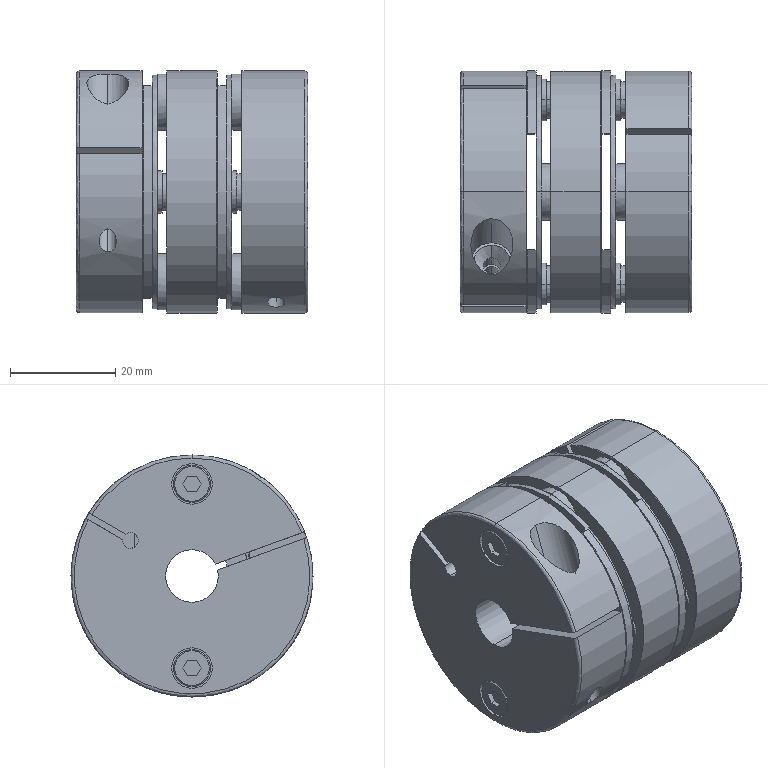Part | SolidWorks | features BaseBody 1 | 1 solid | 200 faces | box 44 x 46 x 46 mm | volume 54630 mm3 | cylinder 87 | plane 82 | cone 24 | spline 7 | commonest cylinder face diameters 7 x16 46 x13 8 x12 3.242 x8 7.7 x8 10.7 x8